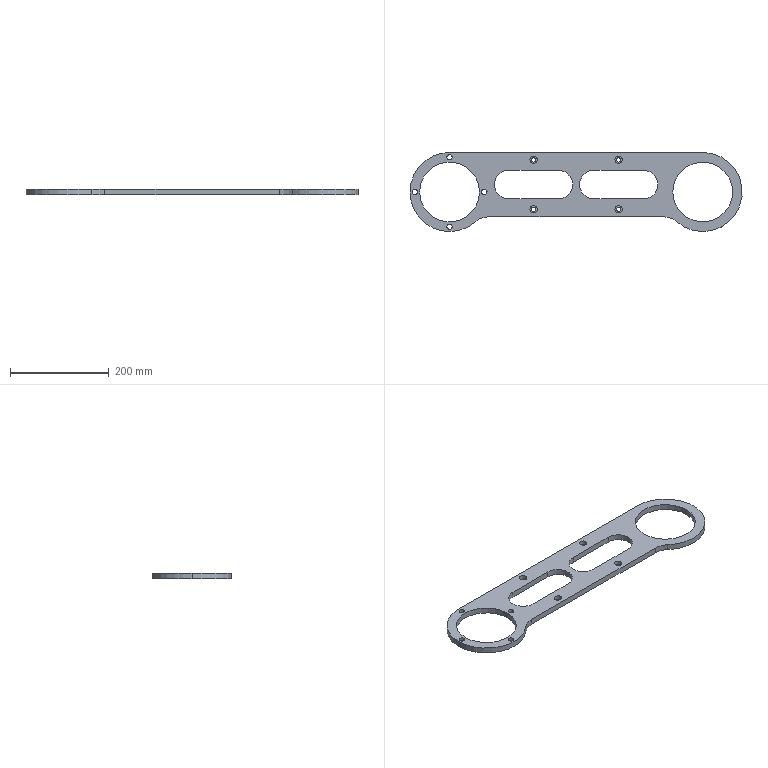Part | SolidWorks | features ICE 4, Extrusion 1, HoleWzd 1 | 1 solid | 51 faces | box 672 x 160 x 12 mm | volume 581826 mm3 | cylinder 39 | plane 12 | commonest cylinder face diameters 9 x8 11 x8 15 x8 58 x6 121 x4 160 x3